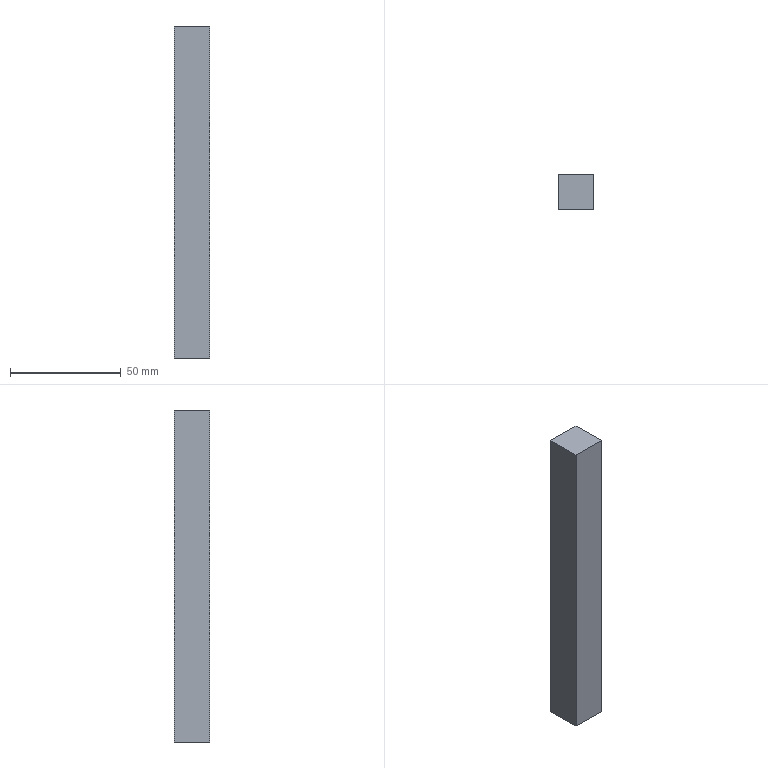Part | SolidWorks | features Extrusion 1 | 1 solid | 6 faces | box 16 x 16 x 150 mm | volume 38400 mm3 | plane 6
STEP:
#1=CARTESIAN_POINT('',(-8.,8.,0.));
#2=VERTEX_POINT('',#1);
#3=CARTESIAN_POINT('',(-8.,-8.,0.));
#4=VERTEX_POINT('',#3);
#5=CARTESIAN_POINT('',(-8.,8.,0.));
#6=DIRECTION('',(0.,-1.,0.));
#7=VECTOR('',#6,1000.);
#8=LINE('',#5,#7);
#9=EDGE_CURVE('',#2,#4,#8,.T.);
#10=ORIENTED_EDGE('',*,*,#9,.T.);
#11=CARTESIAN_POINT('',(-8.,-8.,150.));
#12=VERTEX_POINT('',#11);
#13=CARTESIAN_POINT('',(-8.,-8.,150.));
#14=DIRECTION('',(0.,0.,-1.));
#15=VECTOR('',#14,1000.);
#16=LINE('',#13,#15);
#17=EDGE_CURVE('',#12,#4,#16,.T.);
#18=ORIENTED_EDGE('',*,*,#17,.F.);
#19=CARTESIAN_POINT('',(-8.,8.,150.));
#20=VERTEX_POINT('',#19);
#21=CARTESIAN_POINT('',(-8.,8.,150.));
#22=DIRECTION('',(0.,-1.,0.));
#23=VECTOR('',#22,1000.);
#24=LINE('',#21,#23);
#25=EDGE_CURVE('',#20,#12,#24,.T.);
#26=ORIENTED_EDGE('',*,*,#25,.F.);
#27=CARTESIAN_POINT('',(-8.,8.,150.));
#28=DIRECTION('',(0.,0.,-1.));
#29=VECTOR('',#28,1000.);
#30=LINE('',#27,#29);
#31=EDGE_CURVE('',#20,#2,#30,.T.);
#32=ORIENTED_EDGE('',*,*,#31,.T.);
#33=EDGE_LOOP('',(#10,#18,#26,#32));
#34=FACE_OUTER_BOUND('',#33,.T.);
#35=CARTESIAN_POINT('',(-8.,8.,150.));
#36=DIRECTION('',(1.,0.,0.));
#37=DIRECTION('',(0.,1.,0.));
#38=AXIS2_PLACEMENT_3D('',#35,#36,#37);
#39=PLANE('',#38);
#40=ADVANCED_FACE('',(#34),#39,.F.);
#41=CARTESIAN_POINT('',(8.,-8.,0.));
#42=VERTEX_POINT('',#41);
#43=CARTESIAN_POINT('',(8.,-8.,0.));
#44=DIRECTION('',(1.,0.,0.));
#45=VECTOR('',#44,1000.);
#46=LINE('',#43,#45);
#47=EDGE_CURVE('',#4,#42,#46,.T.);
#48=ORIENTED_EDGE('',*,*,#47,.T.);
#49=CARTESIAN_POINT('',(8.,-8.,150.));
#50=VERTEX_POINT('',#49);
#51=CARTESIAN_POINT('',(8.,-8.,150.));
#52=DIRECTION('',(0.,0.,-1.));
#53=VECTOR('',#52,1000.);
#54=LINE('',#51,#53);
#55=EDGE_CURVE('',#50,#42,#54,.T.);
#56=ORIENTED_EDGE('',*,*,#55,.F.);
#57=CARTESIAN_POINT('',(8.,-8.,150.));
#58=DIRECTION('',(1.,0.,0.));
#59=VECTOR('',#58,1000.);
#60=LINE('',#57,#59);
#61=EDGE_CURVE('',#12,#50,#60,.T.);
#62=ORIENTED_EDGE('',*,*,#61,.F.);
#63=ORIENTED_EDGE('',*,*,#17,.T.);
#64=EDGE_LOOP('',(#48,#56,#62,#63));
#65=FACE_OUTER_BOUND('',#64,.T.);
#66=CARTESIAN_POINT('',(8.,-8.,150.));
#67=DIRECTION('',(0.,1.,0.));
#68=DIRECTION('',(-1.,0.,0.));
#69=AXIS2_PLACEMENT_3D('',#66,#67,#68);
#70=PLANE('',#69);
#71=ADVANCED_FACE('',(#65),#70,.F.);
#72=CARTESIAN_POINT('',(8.,8.,0.));
#73=VERTEX_POINT('',#72);
#74=CARTESIAN_POINT('',(8.,8.,0.));
#75=DIRECTION('',(0.,1.,0.));
#76=VECTOR('',#75,1000.);
#77=LINE('',#74,#76);
#78=EDGE_CURVE('',#42,#73,#77,.T.);
#79=ORIENTED_EDGE('',*,*,#78,.T.);
#80=CARTESIAN_POINT('',(8.,8.,150.));
#81=VERTEX_POINT('',#80);
#82=CARTESIAN_POINT('',(8.,8.,150.));
#83=DIRECTION('',(0.,0.,-1.));
#84=VECTOR('',#83,1000.);
#85=LINE('',#82,#84);
#86=EDGE_CURVE('',#81,#73,#85,.T.);
#87=ORIENTED_EDGE('',*,*,#86,.F.);
#88=CARTESIAN_POINT('',(8.,8.,150.));
#89=DIRECTION('',(0.,1.,0.));
#90=VECTOR('',#89,1000.);
#91=LINE('',#88,#90);
#92=EDGE_CURVE('',#50,#81,#91,.T.);
#93=ORIENTED_EDGE('',*,*,#92,.F.);
#94=ORIENTED_EDGE('',*,*,#55,.T.);
#95=EDGE_LOOP('',(#79,#87,#93,#94));
#96=FACE_OUTER_BOUND('',#95,.T.);
#97=CARTESIAN_POINT('',(8.,8.,150.));
#98=DIRECTION('',(-1.,0.,0.));
#99=DIRECTION('',(0.,-1.,0.));
#100=AXIS2_PLACEMENT_3D('',#97,#98,#99);
#101=PLANE('',#100);
#102=ADVANCED_FACE('',(#96),#101,.F.);
#103=CARTESIAN_POINT('',(8.,8.,0.));
#104=DIRECTION('',(-1.,0.,0.));
#105=VECTOR('',#104,1000.);
#106=LINE('',#103,#105);
#107=EDGE_CURVE('',#73,#2,#106,.T.);
#108=ORIENTED_EDGE('',*,*,#107,.T.);
#109=ORIENTED_EDGE('',*,*,#31,.F.);
#110=CARTESIAN_POINT('',(8.,8.,150.));
#111=DIRECTION('',(-1.,0.,0.));
#112=VECTOR('',#111,1000.);
#113=LINE('',#110,#112);
#114=EDGE_CURVE('',#81,#20,#113,.T.);
#115=ORIENTED_EDGE('',*,*,#114,.F.);
#116=ORIENTED_EDGE('',*,*,#86,.T.);
#117=EDGE_LOOP('',(#108,#109,#115,#116));
#118=FACE_OUTER_BOUND('',#117,.T.);
#119=CARTESIAN_POINT('',(8.,8.,150.));
#120=DIRECTION('',(0.,-1.,0.));
#121=DIRECTION('',(1.,0.,0.));
#122=AXIS2_PLACEMENT_3D('',#119,#120,#121);
#123=PLANE('',#122);
#124=ADVANCED_FACE('',(#118),#123,.F.);
#125=ORIENTED_EDGE('',*,*,#25,.T.);
#126=ORIENTED_EDGE('',*,*,#61,.T.);
#127=ORIENTED_EDGE('',*,*,#92,.T.);
#128=ORIENTED_EDGE('',*,*,#114,.T.);
#129=EDGE_LOOP('',(#125,#126,#127,#128));
#130=FACE_OUTER_BOUND('',#129,.T.);
#131=CARTESIAN_POINT('',(0.,0.,150.));
#132=DIRECTION('',(0.,0.,-1.));
#133=DIRECTION('',(-1.,0.,0.));
#134=AXIS2_PLACEMENT_3D('',#131,#132,#133);
#135=PLANE('',#134);
#136=ADVANCED_FACE('',(#130),#135,.F.);
#137=ORIENTED_EDGE('',*,*,#9,.F.);
#138=ORIENTED_EDGE('',*,*,#107,.F.);
#139=ORIENTED_EDGE('',*,*,#78,.F.);
#140=ORIENTED_EDGE('',*,*,#47,.F.);
#141=EDGE_LOOP('',(#137,#138,#139,#140));
#142=FACE_OUTER_BOUND('',#141,.T.);
#143=CARTESIAN_POINT('',(0.,0.,0.));
#144=DIRECTION('',(0.,0.,-1.));
#145=DIRECTION('',(-1.,0.,0.));
#146=AXIS2_PLACEMENT_3D('',#143,#144,#145);
#147=PLANE('',#146);
#148=ADVANCED_FACE('',(#142),#147,.T.);
#149=CLOSED_SHELL('',(#40,#71,#102,#124,#136,#148));
#150=MANIFOLD_SOLID_BREP('',#149);
#151=CARTESIAN_POINT('',(0.,0.,0.));
#152=DIRECTION('',(0.,0.,1.));
#153=DIRECTION('',(1.,0.,0.));
#154=AXIS2_PLACEMENT_3D('',#151,#152,#153);
#155=(LENGTH_UNIT()NAMED_UNIT(*)SI_UNIT(.MILLI.,.METRE.));
#156=UNCERTAINTY_MEASURE_WITH_UNIT(LENGTH_MEASURE(0.00001),#155,'','');
#157=(NAMED_UNIT(*)PLANE_ANGLE_UNIT()SI_UNIT($,.RADIAN.));
#158=(NAMED_UNIT(*)SI_UNIT($,.STERADIAN.)SOLID_ANGLE_UNIT());
#159=(GEOMETRIC_REPRESENTATION_CONTEXT(3)GLOBAL_UNCERTAINTY_ASSIGNED_CONTEXT((#156))GLOBAL_UNIT_ASSIGNED_CONTEXT((#155,#157,#158))REPRESENTATION_CONTEXT('',''));
#160=ADVANCED_BREP_SHAPE_REPRESENTATION('',(#150,#154),#159);